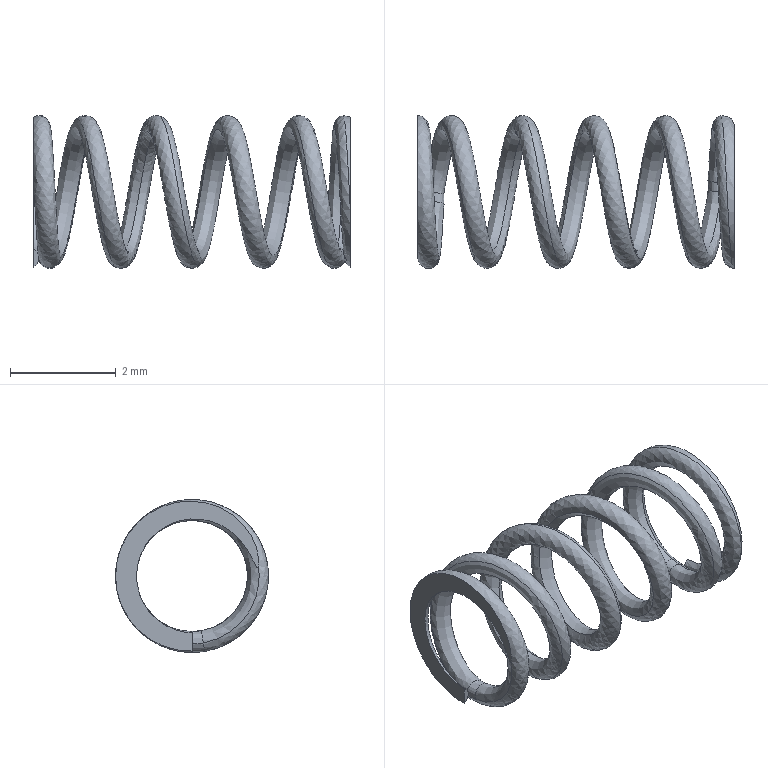Part | SolidWorks | features BaseBody 1 | 1 solid | 14 faces | box 6 x 2.898 x 2.899 mm | volume 5.411 mm3 | spline 10 | plane 4